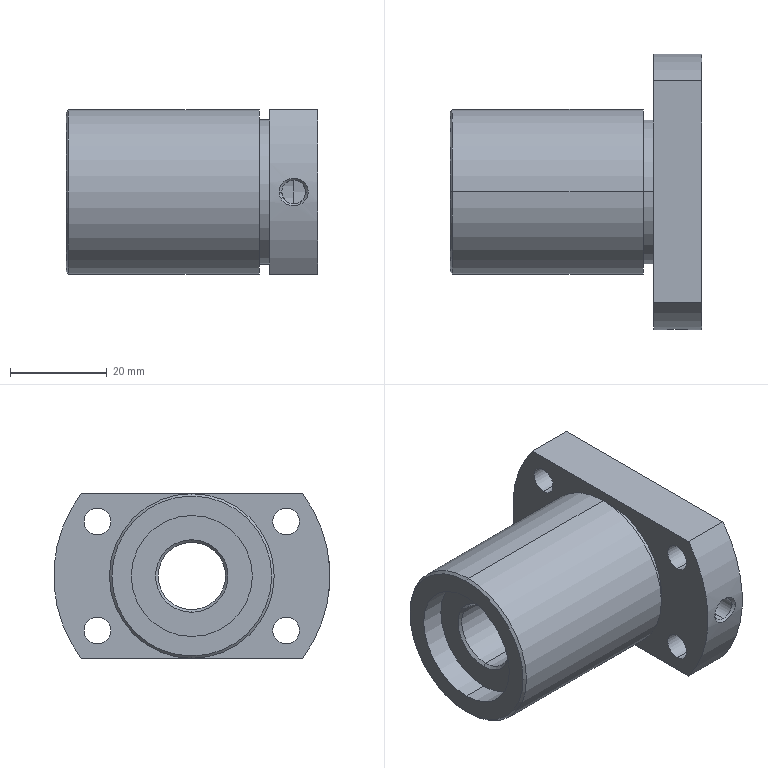Part | SolidWorks | features BaseBody 1 | 1 solid | 41 faces | box 52 x 57 x 34 mm | volume 42280 mm3 | cylinder 24 | plane 9 | cone 8 | commonest cylinder face diameters 5.5 x8 25 x4 4.917 x2 13.917 x2 21 x2 29.8 x2
STEP:
#1=CARTESIAN_POINT('',(39.9,0.,17.));
#2=VERTEX_POINT('',#1);
#3=CARTESIAN_POINT('',(39.9,0.,-17.));
#4=VERTEX_POINT('',#3);
#5=CARTESIAN_POINT('',(39.9,0.,0.));
#6=DIRECTION('',(-1.,0.,0.));
#7=DIRECTION('',(0.,0.,1.));
#8=AXIS2_PLACEMENT_3D('',#5,#6,#7);
#9=CIRCLE('',#8,17.);
#10=EDGE_CURVE('',#2,#4,#9,.T.);
#11=ORIENTED_EDGE('',*,*,#10,.T.);
#12=CARTESIAN_POINT('',(0.5,0.,-17.));
#13=VERTEX_POINT('',#12);
#14=CARTESIAN_POINT('',(42.,0.,-17.));
#15=DIRECTION('',(-1.,0.,0.));
#16=VECTOR('',#15,1000.);
#17=LINE('',#14,#16);
#18=EDGE_CURVE('',#4,#13,#17,.T.);
#19=ORIENTED_EDGE('',*,*,#18,.T.);
#20=CARTESIAN_POINT('',(0.5,0.,17.));
#21=VERTEX_POINT('',#20);
#22=CARTESIAN_POINT('',(0.5,0.,0.));
#23=DIRECTION('',(1.,0.,0.));
#24=DIRECTION('',(0.,0.,1.));
#25=AXIS2_PLACEMENT_3D('',#22,#23,#24);
#26=CIRCLE('',#25,17.);
#27=EDGE_CURVE('',#13,#21,#26,.T.);
#28=ORIENTED_EDGE('',*,*,#27,.T.);
#29=CARTESIAN_POINT('',(42.,0.,17.));
#30=DIRECTION('',(-1.,0.,0.));
#31=VECTOR('',#30,1000.);
#32=LINE('',#29,#31);
#33=EDGE_CURVE('',#2,#21,#32,.T.);
#34=ORIENTED_EDGE('',*,*,#33,.F.);
#35=EDGE_LOOP('',(#11,#19,#28,#34));
#36=FACE_OUTER_BOUND('',#35,.T.);
#37=CARTESIAN_POINT('',(42.,0.,0.));
#38=DIRECTION('',(-1.,0.,0.));
#39=DIRECTION('',(0.,0.,1.));
#40=AXIS2_PLACEMENT_3D('',#37,#38,#39);
#41=CYLINDRICAL_SURFACE('',#40,17.);
#42=ADVANCED_FACE('',(#36),#41,.T.);
#43=CARTESIAN_POINT('',(0.,0.,-16.5));
#44=VERTEX_POINT('',#43);
#45=CARTESIAN_POINT('',(0.,0.,16.5));
#46=VERTEX_POINT('',#45);
#47=CARTESIAN_POINT('',(0.,0.,0.));
#48=DIRECTION('',(1.,0.,0.));
#49=DIRECTION('',(0.,0.,-1.));
#50=AXIS2_PLACEMENT_3D('',#47,#48,#49);
#51=CIRCLE('',#50,16.5);
#52=EDGE_CURVE('',#44,#46,#51,.T.);
#53=ORIENTED_EDGE('',*,*,#52,.T.);
#54=CARTESIAN_POINT('',(0.5,0.,17.));
#55=DIRECTION('',(0.7071,0.,0.7071));
#56=VECTOR('',#55,1000.);
#57=LINE('',#54,#56);
#58=EDGE_CURVE('',#46,#21,#57,.T.);
#59=ORIENTED_EDGE('',*,*,#58,.T.);
#60=ORIENTED_EDGE('',*,*,#27,.F.);
#61=CARTESIAN_POINT('',(0.5,0.,-17.));
#62=DIRECTION('',(0.7071,0.,-0.7071));
#63=VECTOR('',#62,1000.);
#64=LINE('',#61,#63);
#65=EDGE_CURVE('',#44,#13,#64,.T.);
#66=ORIENTED_EDGE('',*,*,#65,.F.);
#67=EDGE_LOOP('',(#53,#59,#60,#66));
#68=FACE_OUTER_BOUND('',#67,.T.);
#69=CARTESIAN_POINT('',(0.5,0.,0.));
#70=DIRECTION('',(1.,0.,0.));
#71=DIRECTION('',(0.,0.,-1.));
#72=AXIS2_PLACEMENT_3D('',#69,#70,#71);
#73=CONICAL_SURFACE('',#72,17.,0.7854);
#74=ADVANCED_FACE('',(#68),#73,.T.);
#75=CARTESIAN_POINT('',(42.,0.,14.9));
#76=VERTEX_POINT('',#75);
#77=CARTESIAN_POINT('',(42.,0.,-14.9));
#78=VERTEX_POINT('',#77);
#79=CARTESIAN_POINT('',(42.,0.,0.));
#80=DIRECTION('',(-1.,0.,0.));
#81=DIRECTION('',(0.,0.,1.));
#82=AXIS2_PLACEMENT_3D('',#79,#80,#81);
#83=CIRCLE('',#82,14.9);
#84=EDGE_CURVE('',#76,#78,#83,.T.);
#85=ORIENTED_EDGE('',*,*,#84,.T.);
#86=CARTESIAN_POINT('',(39.9,0.,-14.9));
#87=VERTEX_POINT('',#86);
#88=CARTESIAN_POINT('',(42.,0.,-14.9));
#89=DIRECTION('',(-1.,0.,0.));
#90=VECTOR('',#89,1000.);
#91=LINE('',#88,#90);
#92=EDGE_CURVE('',#78,#87,#91,.T.);
#93=ORIENTED_EDGE('',*,*,#92,.T.);
#94=CARTESIAN_POINT('',(39.9,0.,14.9));
#95=VERTEX_POINT('',#94);
#96=CARTESIAN_POINT('',(39.9,0.,0.));
#97=DIRECTION('',(1.,0.,0.));
#98=DIRECTION('',(0.,0.,1.));
#99=AXIS2_PLACEMENT_3D('',#96,#97,#98);
#100=CIRCLE('',#99,14.9);
#101=EDGE_CURVE('',#87,#95,#100,.T.);
#102=ORIENTED_EDGE('',*,*,#101,.T.);
#103=CARTESIAN_POINT('',(42.,0.,14.9));
#104=DIRECTION('',(-1.,0.,0.));
#105=VECTOR('',#104,1000.);
#106=LINE('',#103,#105);
#107=EDGE_CURVE('',#76,#95,#106,.T.);
#108=ORIENTED_EDGE('',*,*,#107,.F.);
#109=EDGE_LOOP('',(#85,#93,#102,#108));
#110=FACE_OUTER_BOUND('',#109,.T.);
#111=CARTESIAN_POINT('',(42.,0.,0.));
#112=DIRECTION('',(-1.,0.,0.));
#113=DIRECTION('',(0.,0.,1.));
#114=AXIS2_PLACEMENT_3D('',#111,#112,#113);
#115=CYLINDRICAL_SURFACE('',#114,14.9);
#116=ADVANCED_FACE('',(#110),#115,.T.);
#117=CARTESIAN_POINT('',(5.,0.,-12.5));
#118=VERTEX_POINT('',#117);
#119=CARTESIAN_POINT('',(5.,0.,12.5));
#120=VERTEX_POINT('',#119);
#121=CARTESIAN_POINT('',(5.,0.,0.));
#122=DIRECTION('',(-1.,0.,0.));
#123=DIRECTION('',(0.,0.,1.));
#124=AXIS2_PLACEMENT_3D('',#121,#122,#123);
#125=CIRCLE('',#124,12.5);
#126=EDGE_CURVE('',#118,#120,#125,.T.);
#127=ORIENTED_EDGE('',*,*,#126,.F.);
#128=CARTESIAN_POINT('',(0.,0.,-12.5));
#129=VERTEX_POINT('',#128);
#130=CARTESIAN_POINT('',(52.,0.,-12.5));
#131=DIRECTION('',(-1.,0.,0.));
#132=VECTOR('',#131,1000.);
#133=LINE('',#130,#132);
#134=EDGE_CURVE('',#118,#129,#133,.T.);
#135=ORIENTED_EDGE('',*,*,#134,.T.);
#136=CARTESIAN_POINT('',(0.,0.,12.5));
#137=VERTEX_POINT('',#136);
#138=CARTESIAN_POINT('',(0.,0.,0.));
#139=DIRECTION('',(-1.,0.,0.));
#140=DIRECTION('',(0.,0.,1.));
#141=AXIS2_PLACEMENT_3D('',#138,#139,#140);
#142=CIRCLE('',#141,12.5);
#143=EDGE_CURVE('',#129,#137,#142,.T.);
#144=ORIENTED_EDGE('',*,*,#143,.T.);
#145=CARTESIAN_POINT('',(52.,0.,12.5));
#146=DIRECTION('',(-1.,0.,0.));
#147=VECTOR('',#146,1000.);
#148=LINE('',#145,#147);
#149=EDGE_CURVE('',#120,#137,#148,.T.);
#150=ORIENTED_EDGE('',*,*,#149,.F.);
#151=EDGE_LOOP('',(#127,#135,#144,#150));
#152=FACE_OUTER_BOUND('',#151,.T.);
#153=CARTESIAN_POINT('',(52.,0.,0.));
#154=DIRECTION('',(-1.,0.,0.));
#155=DIRECTION('',(0.,0.,1.));
#156=AXIS2_PLACEMENT_3D('',#153,#154,#155);
#157=CYLINDRICAL_SURFACE('',#156,12.5);
#158=ADVANCED_FACE('',(#152),#157,.F.);
#159=CARTESIAN_POINT('',(52.,19.486,8.5));
#160=VERTEX_POINT('',#159);
#161=CARTESIAN_POINT('',(52.,19.486,14.));
#162=VERTEX_POINT('',#161);
#163=CARTESIAN_POINT('',(52.,19.486,11.25));
#164=DIRECTION('',(-1.,0.,0.));
#165=DIRECTION('',(0.,0.,1.));
#166=AXIS2_PLACEMENT_3D('',#163,#164,#165);
#167=CIRCLE('',#166,2.75);
#168=EDGE_CURVE('',#160,#162,#167,.T.);
#169=ORIENTED_EDGE('',*,*,#168,.F.);
#170=CARTESIAN_POINT('',(42.,19.486,8.5));
#171=VERTEX_POINT('',#170);
#172=CARTESIAN_POINT('',(52.,19.486,8.5));
#173=DIRECTION('',(-1.,0.,0.));
#174=VECTOR('',#173,1000.);
#175=LINE('',#172,#174);
#176=EDGE_CURVE('',#160,#171,#175,.T.);
#177=ORIENTED_EDGE('',*,*,#176,.T.);
#178=CARTESIAN_POINT('',(42.,19.486,14.));
#179=VERTEX_POINT('',#178);
#180=CARTESIAN_POINT('',(42.,19.486,11.25));
#181=DIRECTION('',(-1.,0.,0.));
#182=DIRECTION('',(0.,0.,1.));
#183=AXIS2_PLACEMENT_3D('',#180,#181,#182);
#184=CIRCLE('',#183,2.75);
#185=EDGE_CURVE('',#171,#179,#184,.T.);
#186=ORIENTED_EDGE('',*,*,#185,.T.);
#187=CARTESIAN_POINT('',(52.,19.486,14.));
#188=DIRECTION('',(-1.,0.,0.));
#189=VECTOR('',#188,1000.);
#190=LINE('',#187,#189);
#191=EDGE_CURVE('',#162,#179,#190,.T.);
#192=ORIENTED_EDGE('',*,*,#191,.F.);
#193=EDGE_LOOP('',(#169,#177,#186,#192));
#194=FACE_OUTER_BOUND('',#193,.T.);
#195=CARTESIAN_POINT('',(52.,19.486,11.25));
#196=DIRECTION('',(-1.,0.,0.));
#197=DIRECTION('',(0.,0.,1.));
#198=AXIS2_PLACEMENT_3D('',#195,#196,#197);
#199=CYLINDRICAL_SURFACE('',#198,2.75);
#200=ADVANCED_FACE('',(#194),#199,.F.);
#201=CARTESIAN_POINT('',(52.,-19.486,-14.));
#202=VERTEX_POINT('',#201);
#203=CARTESIAN_POINT('',(52.,-19.486,-8.5));
#204=VERTEX_POINT('',#203);
#205=CARTESIAN_POINT('',(52.,-19.486,-11.25));
#206=DIRECTION('',(-1.,0.,0.));
#207=DIRECTION('',(0.,0.,1.));
#208=AXIS2_PLACEMENT_3D('',#205,#206,#207);
#209=CIRCLE('',#208,2.75);
#210=EDGE_CURVE('',#202,#204,#209,.T.);
#211=ORIENTED_EDGE('',*,*,#210,.F.);
#212=CARTESIAN_POINT('',(42.,-19.486,-14.));
#213=VERTEX_POINT('',#212);
#214=CARTESIAN_POINT('',(52.,-19.486,-14.));
#215=DIRECTION('',(-1.,0.,0.));
#216=VECTOR('',#215,1000.);
#217=LINE('',#214,#216);
#218=EDGE_CURVE('',#202,#213,#217,.T.);
#219=ORIENTED_EDGE('',*,*,#218,.T.);
#220=CARTESIAN_POINT('',(42.,-19.486,-8.5));
#221=VERTEX_POINT('',#220);
#222=CARTESIAN_POINT('',(42.,-19.486,-11.25));
#223=DIRECTION('',(-1.,0.,0.));
#224=DIRECTION('',(0.,0.,1.));
#225=AXIS2_PLACEMENT_3D('',#222,#223,#224);
#226=CIRCLE('',#225,2.75);
#227=EDGE_CURVE('',#213,#221,#226,.T.);
#228=ORIENTED_EDGE('',*,*,#227,.T.);
#229=CARTESIAN_POINT('',(52.,-19.486,-8.5));
#230=DIRECTION('',(-1.,0.,0.));
#231=VECTOR('',#230,1000.);
#232=LINE('',#229,#231);
#233=EDGE_CURVE('',#204,#221,#232,.T.);
#234=ORIENTED_EDGE('',*,*,#233,.F.);
#235=EDGE_LOOP('',(#211,#219,#228,#234));
#236=FACE_OUTER_BOUND('',#235,.T.);
#237=CARTESIAN_POINT('',(52.,-19.486,-11.25));
#238=DIRECTION('',(-1.,0.,0.));
#239=DIRECTION('',(0.,0.,1.));
#240=AXIS2_PLACEMENT_3D('',#237,#238,#239);
#241=CYLINDRICAL_SURFACE('',#240,2.75);
#242=ADVANCED_FACE('',(#236),#241,.F.);
#243=CARTESIAN_POINT('',(52.,19.486,-14.));
#244=VERTEX_POINT('',#243);
#245=CARTESIAN_POINT('',(52.,19.486,-8.5));
#246=VERTEX_POINT('',#245);
#247=CARTESIAN_POINT('',(52.,19.486,-11.25));
#248=DIRECTION('',(-1.,0.,0.));
#249=DIRECTION('',(0.,0.,1.));
#250=AXIS2_PLACEMENT_3D('',#247,#248,#249);
#251=CIRCLE('',#250,2.75);
#252=EDGE_CURVE('',#244,#246,#251,.T.);
#253=ORIENTED_EDGE('',*,*,#252,.F.);
#254=CARTESIAN_POINT('',(42.,19.486,-14.));
#255=VERTEX_POINT('',#254);
#256=CARTESIAN_POINT('',(52.,19.486,-14.));
#257=DIRECTION('',(-1.,0.,0.));
#258=VECTOR('',#257,1000.);
#259=LINE('',#256,#258);
#260=EDGE_CURVE('',#244,#255,#259,.T.);
#261=ORIENTED_EDGE('',*,*,#260,.T.);
#262=CARTESIAN_POINT('',(42.,19.486,-8.5));
#263=VERTEX_POINT('',#262);
#264=CARTESIAN_POINT('',(42.,19.486,-11.25));
#265=DIRECTION('',(-1.,0.,0.));
#266=DIRECTION('',(0.,0.,1.));
#267=AXIS2_PLACEMENT_3D('',#264,#265,#266);
#268=CIRCLE('',#267,2.75);
#269=EDGE_CURVE('',#255,#263,#268,.T.);
#270=ORIENTED_EDGE('',*,*,#269,.T.);
#271=CARTESIAN_POINT('',(52.,19.486,-8.5));
#272=DIRECTION('',(-1.,0.,0.));
#273=VECTOR('',#272,1000.);
#274=LINE('',#271,#273);
#275=EDGE_CURVE('',#246,#263,#274,.T.);
#276=ORIENTED_EDGE('',*,*,#275,.F.);
#277=EDGE_LOOP('',(#253,#261,#270,#276));
#278=FACE_OUTER_BOUND('',#277,.T.);
#279=CARTESIAN_POINT('',(52.,19.486,-11.25));
#280=DIRECTION('',(-1.,0.,0.));
#281=DIRECTION('',(0.,0.,1.));
#282=AXIS2_PLACEMENT_3D('',#279,#280,#281);
#283=CYLINDRICAL_SURFACE('',#282,2.75);
#284=ADVANCED_FACE('',(#278),#283,.F.);
#285=CARTESIAN_POINT('',(52.,-19.486,8.5));
#286=VERTEX_POINT('',#285);
#287=CARTESIAN_POINT('',(52.,-19.486,14.));
#288=VERTEX_POINT('',#287);
#289=CARTESIAN_POINT('',(52.,-19.486,11.25));
#290=DIRECTION('',(-1.,0.,0.));
#291=DIRECTION('',(0.,0.,1.));
#292=AXIS2_PLACEMENT_3D('',#289,#290,#291);
#293=CIRCLE('',#292,2.75);
#294=EDGE_CURVE('',#286,#288,#293,.T.);
#295=ORIENTED_EDGE('',*,*,#294,.F.);
#296=CARTESIAN_POINT('',(42.,-19.486,8.5));
#297=VERTEX_POINT('',#296);
#298=CARTESIAN_POINT('',(52.,-19.486,8.5));
#299=DIRECTION('',(-1.,0.,0.));
#300=VECTOR('',#299,1000.);
#301=LINE('',#298,#300);
#302=EDGE_CURVE('',#286,#297,#301,.T.);
#303=ORIENTED_EDGE('',*,*,#302,.T.);
#304=CARTESIAN_POINT('',(42.,-19.486,14.));
#305=VERTEX_POINT('',#304);
#306=CARTESIAN_POINT('',(42.,-19.486,11.25));
#307=DIRECTION('',(-1.,0.,0.));
#308=DIRECTION('',(0.,0.,1.));
#309=AXIS2_PLACEMENT_3D('',#306,#307,#308);
#310=CIRCLE('',#309,2.75);
#311=EDGE_CURVE('',#297,#305,#310,.T.);
#312=ORIENTED_EDGE('',*,*,#311,.T.);
#313=CARTESIAN_POINT('',(52.,-19.486,14.));
#314=DIRECTION('',(-1.,0.,0.));
#315=VECTOR('',#314,1000.);
#316=LINE('',#313,#315);
#317=EDGE_CURVE('',#288,#305,#316,.T.);
#318=ORIENTED_EDGE('',*,*,#317,.F.);
#319=EDGE_LOOP('',(#295,#303,#312,#318));
#320=FACE_OUTER_BOUND('',#319,.T.);
#321=CARTESIAN_POINT('',(52.,-19.486,11.25));
#322=DIRECTION('',(-1.,0.,0.));
#323=DIRECTION('',(0.,0.,1.));
#324=AXIS2_PLACEMENT_3D('',#321,#322,#323);
#325=CYLINDRICAL_SURFACE('',#324,2.75);
#326=ADVANCED_FACE('',(#320),#325,.F.);
#327=CARTESIAN_POINT('',(5.542,0.,-6.958));
#328=VERTEX_POINT('',#327);
#329=CARTESIAN_POINT('',(5.542,0.,6.958));
#330=VERTEX_POINT('',#329);
#331=CARTESIAN_POINT('',(5.542,0.,0.));
#332=DIRECTION('',(-1.,0.,0.));
#333=DIRECTION('',(0.,0.,1.));
#334=AXIS2_PLACEMENT_3D('',#331,#332,#333);
#335=CIRCLE('',#334,6.958);
#336=EDGE_CURVE('',#328,#330,#335,.T.);
#337=ORIENTED_EDGE('',*,*,#336,.F.);
#338=CARTESIAN_POINT('',(5.,0.,-7.5));
#339=VERTEX_POINT('',#338);
#340=CARTESIAN_POINT('',(5.,0.,-7.5));
#341=DIRECTION('',(-0.7071,0.,-0.7071));
#342=VECTOR('',#341,1000.);
#343=LINE('',#340,#342);
#344=EDGE_CURVE('',#328,#339,#343,.T.);
#345=ORIENTED_EDGE('',*,*,#344,.T.);
#346=CARTESIAN_POINT('',(5.,0.,7.5));
#347=VERTEX_POINT('',#346);
#348=CARTESIAN_POINT('',(5.,0.,0.));
#349=DIRECTION('',(1.,0.,0.));
#350=DIRECTION('',(0.,0.,1.));
#351=AXIS2_PLACEMENT_3D('',#348,#349,#350);
#352=CIRCLE('',#351,7.5);
#353=EDGE_CURVE('',#347,#339,#352,.T.);
#354=ORIENTED_EDGE('',*,*,#353,.F.);
#355=CARTESIAN_POINT('',(5.,0.,7.5));
#356=DIRECTION('',(-0.7071,0.,0.7071));
#357=VECTOR('',#356,1000.);
#358=LINE('',#355,#357);
#359=EDGE_CURVE('',#330,#347,#358,.T.);
#360=ORIENTED_EDGE('',*,*,#359,.F.);
#361=EDGE_LOOP('',(#337,#345,#354,#360));
#362=FACE_OUTER_BOUND('',#361,.T.);
#363=CARTESIAN_POINT('',(5.,0.,0.));
#364=DIRECTION('',(-1.,0.,0.));
#365=DIRECTION('',(0.,0.,1.));
#366=AXIS2_PLACEMENT_3D('',#363,#364,#365);
#367=CONICAL_SURFACE('',#366,7.5,0.7854);
#368=ADVANCED_FACE('',(#362),#367,.F.);
#369=CARTESIAN_POINT('',(44.542,-27.958,0.));
#370=VERTEX_POINT('',#369);
#371=CARTESIAN_POINT('',(47.,-27.958,-2.458));
#372=VERTEX_POINT('',#371);
#373=CARTESIAN_POINT('',(47.,-27.958,0.));
#374=DIRECTION('',(0.,-1.,0.));
#375=DIRECTION('',(0.,0.,-1.));
#376=AXIS2_PLACEMENT_3D('',#373,#374,#375);
#377=CIRCLE('',#376,2.458);
#378=EDGE_CURVE('',#370,#372,#377,.T.);
#379=ORIENTED_EDGE('',*,*,#378,.F.);
#380=CARTESIAN_POINT('',(44.,-28.5,0.));
#381=VERTEX_POINT('',#380);
#382=CARTESIAN_POINT('',(43.997,-28.503,0.));
#383=DIRECTION('',(-0.7071,-0.7071,0.));
#384=VECTOR('',#383,1000.);
#385=LINE('',#382,#384);
#386=EDGE_CURVE('',#370,#381,#385,.T.);
#387=ORIENTED_EDGE('',*,*,#386,.T.);
#388=CARTESIAN_POINT('',(50.,-28.5,0.));
#389=VERTEX_POINT('',#388);
#390=CARTESIAN_POINT('',(50.,-28.5,0.));
#391=CARTESIAN_POINT('',(50.,-28.5,-0.1909));
#392=CARTESIAN_POINT('',(49.98,-28.498,-0.384));
#393=CARTESIAN_POINT('',(49.899,-28.49,-0.7601));
#394=CARTESIAN_POINT('',(49.839,-28.485,-0.9415));
#395=CARTESIAN_POINT('',(49.683,-28.471,-1.292));
#396=CARTESIAN_POINT('',(49.585,-28.463,-1.46));
#397=CARTESIAN_POINT('',(49.362,-28.445,-1.77));
#398=CARTESIAN_POINT('',(49.235,-28.436,-1.914));
#399=CARTESIAN_POINT('',(48.952,-28.417,-2.177));
#400=CARTESIAN_POINT('',(48.8,-28.408,-2.292));
#401=CARTESIAN_POINT('',(48.475,-28.391,-2.494));
#402=CARTESIAN_POINT('',(48.301,-28.383,-2.58));
#403=CARTESIAN_POINT('',(47.943,-28.37,-2.718));
#404=CARTESIAN_POINT('',(47.759,-28.365,-2.769));
#405=CARTESIAN_POINT('',(47.382,-28.358,-2.839));
#406=CARTESIAN_POINT('',(47.188,-28.356,-2.857));
#407=CARTESIAN_POINT('',(46.802,-28.357,-2.856));
#408=CARTESIAN_POINT('',(46.611,-28.358,-2.838));
#409=CARTESIAN_POINT('',(46.237,-28.365,-2.768));
#410=CARTESIAN_POINT('',(46.051,-28.37,-2.716));
#411=CARTESIAN_POINT('',(45.692,-28.383,-2.577));
#412=CARTESIAN_POINT('',(45.521,-28.391,-2.492));
#413=CARTESIAN_POINT('',(45.198,-28.408,-2.29));
#414=CARTESIAN_POINT('',(45.043,-28.417,-2.172));
#415=CARTESIAN_POINT('',(44.763,-28.436,-1.911));
#416=CARTESIAN_POINT('',(44.637,-28.445,-1.769));
#417=CARTESIAN_POINT('',(44.414,-28.463,-1.459));
#418=CARTESIAN_POINT('',(44.316,-28.471,-1.29));
#419=CARTESIAN_POINT('',(44.161,-28.485,-0.9409));
#420=CARTESIAN_POINT('',(44.101,-28.49,-0.7598));
#421=CARTESIAN_POINT('',(44.02,-28.498,-0.3831));
#422=CARTESIAN_POINT('',(44.,-28.5,-0.1908));
#423=CARTESIAN_POINT('',(44.,-28.5,0.));
#424=B_SPLINE_CURVE_WITH_KNOTS('',3,(#390,#391,#392,#393,#394,#395,#396,#397,#398,#399,#400,#401,#402,#403,#404,#405,#406,#407,#408,#409,#410,#411,#412,#413,#414,#415,#416,#417,#418,#419,#420,#421,#422,#423),.UNSPECIFIED.,.F.,.F.,(4,2,2,2,2,2,2,2,2,2,2,2,2,2,2,2,4),(0.01373,0.0143,0.01488,0.01545,0.01602,0.01659,0.01716,0.01774,0.01831,0.01888,0.01945,0.02002,0.0206,0.02117,0.02174,0.02231,0.02288),.UNSPECIFIED.);
#425=EDGE_CURVE('',#389,#381,#424,.T.);
#426=ORIENTED_EDGE('',*,*,#425,.F.);
#427=CARTESIAN_POINT('',(49.458,-27.958,0.));
#428=VERTEX_POINT('',#427);
#429=CARTESIAN_POINT('',(50.003,-28.503,0.));
#430=DIRECTION('',(0.7071,-0.7071,0.));
#431=VECTOR('',#430,1000.);
#432=LINE('',#429,#431);
#433=EDGE_CURVE('',#428,#389,#432,.T.);
#434=ORIENTED_EDGE('',*,*,#433,.F.);
#435=CARTESIAN_POINT('',(47.,-27.958,0.));
#436=DIRECTION('',(0.,-1.,0.));
#437=DIRECTION('',(0.,0.,-1.));
#438=AXIS2_PLACEMENT_3D('',#435,#436,#437);
#439=CIRCLE('',#438,2.458);
#440=EDGE_CURVE('',#372,#428,#439,.T.);
#441=ORIENTED_EDGE('',*,*,#440,.F.);
#442=EDGE_LOOP('',(#379,#387,#426,#434,#441));
#443=FACE_OUTER_BOUND('',#442,.T.);
#444=CARTESIAN_POINT('',(47.,-28.503,0.));
#445=DIRECTION('',(0.,-1.,0.));
#446=DIRECTION('',(1.,0.,0.));
#447=AXIS2_PLACEMENT_3D('',#444,#445,#446);
#448=CONICAL_SURFACE('',#447,3.003,0.7854);
#449=ADVANCED_FACE('',(#443),#448,.F.);
#450=CARTESIAN_POINT('',(41.459,0.,-6.958));
#451=VERTEX_POINT('',#450);
#452=CARTESIAN_POINT('',(41.459,0.,6.958));
#453=VERTEX_POINT('',#452);
#454=CARTESIAN_POINT('',(41.459,0.,0.));
#455=DIRECTION('',(-1.,0.,0.));
#456=DIRECTION('',(0.,0.,1.));
#457=AXIS2_PLACEMENT_3D('',#454,#455,#456);
#458=CIRCLE('',#457,6.958);
#459=EDGE_CURVE('',#451,#453,#458,.T.);
#460=ORIENTED_EDGE('',*,*,#459,.F.);
#461=CARTESIAN_POINT('',(52.,0.,-6.958));
#462=DIRECTION('',(-1.,0.,0.));
#463=VECTOR('',#462,1000.);
#464=LINE('',#461,#463);
#465=EDGE_CURVE('',#451,#328,#464,.T.);
#466=ORIENTED_EDGE('',*,*,#465,.T.);
#467=ORIENTED_EDGE('',*,*,#336,.T.);
#468=CARTESIAN_POINT('',(52.,0.,6.958));
#469=DIRECTION('',(-1.,0.,0.));
#470=VECTOR('',#469,1000.);
#471=LINE('',#468,#470);
#472=EDGE_CURVE('',#453,#330,#471,.T.);
#473=ORIENTED_EDGE('',*,*,#472,.F.);
#474=EDGE_LOOP('',(#460,#466,#467,#473));
#475=FACE_OUTER_BOUND('',#474,.T.);
#476=CARTESIAN_POINT('',(52.,0.,0.));
#477=DIRECTION('',(-1.,0.,0.));
#478=DIRECTION('',(0.,0.,1.));
#479=AXIS2_PLACEMENT_3D('',#476,#477,#478);
#480=CYLINDRICAL_SURFACE('',#479,6.958);
#481=ADVANCED_FACE('',(#475),#480,.F.);
#482=CARTESIAN_POINT('',(52.,0.,-12.5));
#483=VERTEX_POINT('',#482);
#484=CARTESIAN_POINT('',(52.,0.,12.5));
#485=VERTEX_POINT('',#484);
#486=CARTESIAN_POINT('',(52.,0.,0.));
#487=DIRECTION('',(-1.,0.,0.));
#488=DIRECTION('',(0.,0.,1.));
#489=AXIS2_PLACEMENT_3D('',#486,#487,#488);
#490=CIRCLE('',#489,12.5);
#491=EDGE_CURVE('',#483,#485,#490,.T.);
#492=ORIENTED_EDGE('',*,*,#491,.F.);
#493=CARTESIAN_POINT('',(47.,0.,-12.5));
#494=VERTEX_POINT('',#493);
#495=CARTESIAN_POINT('',(52.,0.,-12.5));
#496=DIRECTION('',(-1.,0.,0.));
#497=VECTOR('',#496,1000.);
#498=LINE('',#495,#497);
#499=EDGE_CURVE('',#483,#494,#498,.T.);
#500=ORIENTED_EDGE('',*,*,#499,.T.);
#501=CARTESIAN_POINT('',(47.,-12.256,-2.459));
#502=VERTEX_POINT('',#501);
#503=CARTESIAN_POINT('',(47.,0.,0.));
#504=DIRECTION('',(1.,0.,0.));
#505=DIRECTION('',(0.,0.,1.));
#506=AXIS2_PLACEMENT_3D('',#503,#504,#505);
#507=CIRCLE('',#506,12.5);
#508=EDGE_CURVE('',#502,#494,#507,.T.);
#509=ORIENTED_EDGE('',*,*,#508,.F.);
#510=CARTESIAN_POINT('',(47.,-12.256,2.459));
#511=VERTEX_POINT('',#510);
#512=CARTESIAN_POINT('',(47.,-12.256,2.459));
#513=CARTESIAN_POINT('',(47.163,-12.256,2.459));
#514=CARTESIAN_POINT('',(47.323,-12.259,2.442));
#515=CARTESIAN_POINT('',(47.638,-12.271,2.38));
#516=CARTESIAN_POINT('',(47.794,-12.281,2.332));
#517=CARTESIAN_POINT('',(48.091,-12.303,2.209));
#518=CARTESIAN_POINT('',(48.232,-12.317,2.133));
#519=CARTESIAN_POINT('',(48.499,-12.347,1.955));
#520=CARTESIAN_POINT('',(48.625,-12.363,1.851));
#521=CARTESIAN_POINT('',(48.965,-12.41,1.512));
#522=CARTESIAN_POINT('',(49.148,-12.442,1.239));
#523=CARTESIAN_POINT('',(49.332,-12.476,0.7953));
#524=CARTESIAN_POINT('',(49.379,-12.485,0.64));
#525=CARTESIAN_POINT('',(49.443,-12.497,0.3225));
#526=CARTESIAN_POINT('',(49.458,-12.5,0.1627));
#527=CARTESIAN_POINT('',(49.459,-12.5,-0.1588));
#528=CARTESIAN_POINT('',(49.443,-12.497,-0.3221));
#529=CARTESIAN_POINT('',(49.38,-12.485,-0.6377));
#530=CARTESIAN_POINT('',(49.333,-12.476,-0.7911));
#531=CARTESIAN_POINT('',(49.21,-12.453,-1.089));
#532=CARTESIAN_POINT('',(49.133,-12.44,-1.233));
#533=CARTESIAN_POINT('',(48.956,-12.411,-1.499));
#534=CARTESIAN_POINT('',(48.854,-12.395,-1.623));
#535=CARTESIAN_POINT('',(48.625,-12.363,-1.852));
#536=CARTESIAN_POINT('',(48.501,-12.347,-1.953));
#537=CARTESIAN_POINT('',(48.236,-12.317,-2.131));
#538=CARTESIAN_POINT('',(48.092,-12.303,-2.209));
#539=CARTESIAN_POINT('',(47.795,-12.281,-2.332));
#540=CARTESIAN_POINT('',(47.642,-12.272,-2.379));
#541=CARTESIAN_POINT('',(47.326,-12.259,-2.442));
#542=CARTESIAN_POINT('',(47.163,-12.256,-2.459));
#543=CARTESIAN_POINT('',(47.,-12.256,-2.459));
#544=B_SPLINE_CURVE_WITH_KNOTS('',3,(#512,#513,#514,#515,#516,#517,#518,#519,#520,#521,#522,#523,#524,#525,#526,#527,#528,#529,#530,#531,#532,#533,#534,#535,#536,#537,#538,#539,#540,#541,#542,#543),.UNSPECIFIED.,.F.,.F.,(4,2,2,2,2,2,2,2,2,2,2,2,2,2,2,4),(0.,0.0004814,0.0009629,0.001444,0.001926,0.002889,0.00337,0.003852,0.004333,0.004814,0.005296,0.005777,0.006259,0.00674,0.007222,0.007703),.UNSPECIFIED.);
#545=EDGE_CURVE('',#511,#502,#544,.T.);
#546=ORIENTED_EDGE('',*,*,#545,.F.);
#547=CARTESIAN_POINT('',(47.,0.,12.5));
#548=VERTEX_POINT('',#547);
#549=CARTESIAN_POINT('',(47.,0.,0.));
#550=DIRECTION('',(1.,0.,0.));
#551=DIRECTION('',(0.,0.,1.));
#552=AXIS2_PLACEMENT_3D('',#549,#550,#551);
#553=CIRCLE('',#552,12.5);
#554=EDGE_CURVE('',#548,#511,#553,.T.);
#555=ORIENTED_EDGE('',*,*,#554,.F.);
#556=CARTESIAN_POINT('',(52.,0.,12.5));
#557=DIRECTION('',(-1.,0.,0.));
#558=VECTOR('',#557,1000.);
#559=LINE('',#556,#558);
#560=EDGE_CURVE('',#485,#548,#559,.T.);
#561=ORIENTED_EDGE('',*,*,#560,.F.);
#562=EDGE_LOOP('',(#492,#500,#509,#546,#555,#561));
#563=FACE_OUTER_BOUND('',#562,.T.);
#564=CARTESIAN_POINT('',(52.,0.,0.));
#565=DIRECTION('',(-1.,0.,0.));
#566=DIRECTION('',(0.,0.,1.));
#567=AXIS2_PLACEMENT_3D('',#564,#565,#566);
#568=CYLINDRICAL_SURFACE('',#567,12.5);
#569=ADVANCED_FACE('',(#563),#568,.F.);
#570=CARTESIAN_POINT('',(47.,-27.958,2.458));
#571=VERTEX_POINT('',#570);
#572=CARTESIAN_POINT('',(47.,-27.958,0.));
#573=DIRECTION('',(0.,-1.,0.));
#574=DIRECTION('',(0.,0.,-1.));
#575=AXIS2_PLACEMENT_3D('',#572,#573,#574);
#576=CIRCLE('',#575,2.458);
#577=EDGE_CURVE('',#571,#370,#576,.T.);
#578=ORIENTED_EDGE('',*,*,#577,.T.);
#579=ORIENTED_EDGE('',*,*,#378,.T.);
#580=CARTESIAN_POINT('',(47.,-28.5,-2.459));
#581=DIRECTION('',(0.,1.,0.));
#582=VECTOR('',#581,1000.);
#583=LINE('',#580,#582);
#584=EDGE_CURVE('',#372,#502,#583,.T.);
#585=ORIENTED_EDGE('',*,*,#584,.T.);
#586=CARTESIAN_POINT('',(47.,-10.208,-2.459));
#587=VERTEX_POINT('',#586);
#588=CARTESIAN_POINT('',(47.,-28.5,-2.459));
#589=DIRECTION('',(0.,-1.,0.));
#590=VECTOR('',#589,1000.);
#591=LINE('',#588,#590);
#592=EDGE_CURVE('',#587,#502,#591,.T.);
#593=ORIENTED_EDGE('',*,*,#592,.F.);
#594=CARTESIAN_POINT('',(47.,-10.208,2.459));
#595=VERTEX_POINT('',#594);
#596=CARTESIAN_POINT('',(47.,-10.208,2.459));
#597=CARTESIAN_POINT('',(46.837,-10.208,2.459));
#598=CARTESIAN_POINT('',(46.677,-10.212,2.442));
#599=CARTESIAN_POINT('',(46.362,-10.227,2.38));
#600=CARTESIAN_POINT('',(46.206,-10.238,2.332));
#601=CARTESIAN_POINT('',(45.908,-10.265,2.209));
#602=CARTESIAN_POINT('',(45.767,-10.281,2.133));
#603=CARTESIAN_POINT('',(45.5,-10.317,1.955));
#604=CARTESIAN_POINT('',(45.375,-10.336,1.851));
#605=CARTESIAN_POINT('',(45.036,-10.393,1.513));
#606=CARTESIAN_POINT('',(44.853,-10.431,1.239));
#607=CARTESIAN_POINT('',(44.668,-10.471,0.796));
#608=CARTESIAN_POINT('',(44.621,-10.482,0.6405));
#609=CARTESIAN_POINT('',(44.557,-10.496,0.3229));
#610=CARTESIAN_POINT('',(44.542,-10.5,0.1631));
#611=CARTESIAN_POINT('',(44.541,-10.5,-0.1588));
#612=CARTESIAN_POINT('',(44.557,-10.496,-0.3223));
#613=CARTESIAN_POINT('',(44.62,-10.482,-0.6381));
#614=CARTESIAN_POINT('',(44.667,-10.471,-0.7916));
#615=CARTESIAN_POINT('',(44.852,-10.431,-1.239));
#616=CARTESIAN_POINT('',(45.033,-10.393,-1.51));
#617=CARTESIAN_POINT('',(45.375,-10.336,-1.852));
#618=CARTESIAN_POINT('',(45.498,-10.317,-1.953));
#619=CARTESIAN_POINT('',(45.764,-10.282,-2.131));
#620=CARTESIAN_POINT('',(45.908,-10.265,-2.208));
#621=CARTESIAN_POINT('',(46.204,-10.238,-2.332));
#622=CARTESIAN_POINT('',(46.358,-10.227,-2.379));
#623=CARTESIAN_POINT('',(46.674,-10.212,-2.442));
#624=CARTESIAN_POINT('',(46.837,-10.208,-2.459));
#625=CARTESIAN_POINT('',(47.,-10.208,-2.459));
#626=B_SPLINE_CURVE_WITH_KNOTS('',3,(#596,#597,#598,#599,#600,#601,#602,#603,#604,#605,#606,#607,#608,#609,#610,#611,#612,#613,#614,#615,#616,#617,#618,#619,#620,#621,#622,#623,#624,#625),.UNSPECIFIED.,.F.,.F.,(4,2,2,2,2,2,2,2,2,2,2,2,2,2,4),(0.,0.0004819,0.0009639,0.001446,0.001928,0.002892,0.003374,0.003855,0.004337,0.004819,0.005783,0.006265,0.006747,0.007229,0.007711),.UNSPECIFIED.);
#627=EDGE_CURVE('',#595,#587,#626,.T.);
#628=ORIENTED_EDGE('',*,*,#627,.F.);
#629=CARTESIAN_POINT('',(47.,-28.5,2.459));
#630=DIRECTION('',(0.,1.,0.));
#631=VECTOR('',#630,1000.);
#632=LINE('',#629,#631);
#633=EDGE_CURVE('',#511,#595,#632,.T.);
#634=ORIENTED_EDGE('',*,*,#633,.F.);
#635=CARTESIAN_POINT('',(47.,-28.5,2.459));
#636=DIRECTION('',(0.,1.,0.));
#637=VECTOR('',#636,1000.);
#638=LINE('',#635,#637);
#639=EDGE_CURVE('',#571,#511,#638,.T.);
#640=ORIENTED_EDGE('',*,*,#639,.F.);
#641=EDGE_LOOP('',(#578,#579,#585,#593,#628,#634,#640));
#642=FACE_OUTER_BOUND('',#641,.T.);
#643=CARTESIAN_POINT('',(47.,-28.5,0.));
#644=DIRECTION('',(0.,1.,0.));
#645=DIRECTION('',(0.,0.,1.));
#646=AXIS2_PLACEMENT_3D('',#643,#644,#645);
#647=CYLINDRICAL_SURFACE('',#646,2.459);
#648=ADVANCED_FACE('',(#642),#647,.F.);
#649=ORIENTED_EDGE('',*,*,#459,.T.);
#650=CARTESIAN_POINT('',(42.,0.,7.5));
#651=VERTEX_POINT('',#650);
#652=CARTESIAN_POINT('',(42.,0.,7.5));
#653=DIRECTION('',(0.7071,0.,0.7071));
#654=VECTOR('',#653,1000.);
#655=LINE('',#652,#654);
#656=EDGE_CURVE('',#453,#651,#655,.T.);
#657=ORIENTED_EDGE('',*,*,#656,.T.);
#658=CARTESIAN_POINT('',(42.,0.,-7.5));
#659=VERTEX_POINT('',#658);
#660=CARTESIAN_POINT('',(42.,0.,0.));
#661=DIRECTION('',(-1.,0.,0.));
#662=DIRECTION('',(0.,0.,-1.));
#663=AXIS2_PLACEMENT_3D('',#660,#661,#662);
#664=CIRCLE('',#663,7.5);
#665=EDGE_CURVE('',#659,#651,#664,.T.);
#666=ORIENTED_EDGE('',*,*,#665,.F.);
#667=CARTESIAN_POINT('',(42.,0.,-7.5));
#668=DIRECTION('',(0.7071,0.,-0.7071));
#669=VECTOR('',#668,1000.);
#670=LINE('',#667,#669);
#671=EDGE_CURVE('',#451,#659,#670,.T.);
#672=ORIENTED_EDGE('',*,*,#671,.F.);
#673=EDGE_LOOP('',(#649,#657,#666,#672));
#674=FACE_OUTER_BOUND('',#673,.T.);
#675=CARTESIAN_POINT('',(42.,0.,0.));
#676=DIRECTION('',(1.,0.,0.));
#677=DIRECTION('',(0.,0.,-1.));
#678=AXIS2_PLACEMENT_3D('',#675,#676,#677);
#679=CONICAL_SURFACE('',#678,7.5,0.7854);
#680=ADVANCED_FACE('',(#674),#679,.F.);
#681=CARTESIAN_POINT('',(47.,0.,-10.5));
#682=VERTEX_POINT('',#681);
#683=CARTESIAN_POINT('',(47.,0.,0.));
#684=DIRECTION('',(-1.,0.,0.));
#685=DIRECTION('',(0.,0.,1.));
#686=AXIS2_PLACEMENT_3D('',#683,#684,#685);
#687=CIRCLE('',#686,10.5);
#688=EDGE_CURVE('',#682,#587,#687,.T.);
#689=ORIENTED_EDGE('',*,*,#688,.F.);
#690=CARTESIAN_POINT('',(42.,0.,-10.5));
#691=VERTEX_POINT('',#690);
#692=CARTESIAN_POINT('',(52.,0.,-10.5));
#693=DIRECTION('',(-1.,0.,0.));
#694=VECTOR('',#693,1000.);
#695=LINE('',#692,#694);
#696=EDGE_CURVE('',#682,#691,#695,.T.);
#697=ORIENTED_EDGE('',*,*,#696,.T.);
#698=CARTESIAN_POINT('',(42.,0.,10.5));
#699=VERTEX_POINT('',#698);
#700=CARTESIAN_POINT('',(42.,0.,0.));
#701=DIRECTION('',(1.,0.,0.));
#702=DIRECTION('',(0.,0.,1.));
#703=AXIS2_PLACEMENT_3D('',#700,#701,#702);
#704=CIRCLE('',#703,10.5);
#705=EDGE_CURVE('',#699,#691,#704,.T.);
#706=ORIENTED_EDGE('',*,*,#705,.F.);
#707=CARTESIAN_POINT('',(47.,0.,10.5));
#708=VERTEX_POINT('',#707);
#709=CARTESIAN_POINT('',(52.,0.,10.5));
#710=DIRECTION('',(-1.,0.,0.));
#711=VECTOR('',#710,1000.);
#712=LINE('',#709,#711);
#713=EDGE_CURVE('',#708,#699,#712,.T.);
#714=ORIENTED_EDGE('',*,*,#713,.F.);
#715=CARTESIAN_POINT('',(47.,0.,0.));
#716=DIRECTION('',(-1.,0.,0.));
#717=DIRECTION('',(0.,0.,1.));
#718=AXIS2_PLACEMENT_3D('',#715,#716,#717);
#719=CIRCLE('',#718,10.5);
#720=EDGE_CURVE('',#595,#708,#719,.T.);
#721=ORIENTED_EDGE('',*,*,#720,.F.);
#722=ORIENTED_EDGE('',*,*,#627,.T.);
#723=EDGE_LOOP('',(#689,#697,#706,#714,#721,#722));
#724=FACE_OUTER_BOUND('',#723,.T.);
#725=CARTESIAN_POINT('',(52.,0.,0.));
#726=DIRECTION('',(-1.,0.,0.));
#727=DIRECTION('',(0.,0.,1.));
#728=AXIS2_PLACEMENT_3D('',#725,#726,#727);
#729=CYLINDRICAL_SURFACE('',#728,10.5);
#730=ADVANCED_FACE('',(#724),#729,.F.);
#731=ORIENTED_EDGE('',*,*,#18,.F.);
#732=CARTESIAN_POINT('',(39.9,0.,0.));
#733=DIRECTION('',(-1.,0.,0.));
#734=DIRECTION('',(0.,0.,1.));
#735=AXIS2_PLACEMENT_3D('',#732,#733,#734);
#736=CIRCLE('',#735,17.);
#737=EDGE_CURVE('',#4,#2,#736,.T.);
#738=ORIENTED_EDGE('',*,*,#737,.T.);
#739=ORIENTED_EDGE('',*,*,#33,.T.);
#740=CARTESIAN_POINT('',(0.5,0.,0.));
#741=DIRECTION('',(1.,0.,0.));
#742=DIRECTION('',(0.,0.,1.));
#743=AXIS2_PLACEMENT_3D('',#740,#741,#742);
#744=CIRCLE('',#743,17.);
#745=EDGE_CURVE('',#21,#13,#744,.T.);
#746=ORIENTED_EDGE('',*,*,#745,.T.);
#747=EDGE_LOOP('',(#731,#738,#739,#746));
#748=FACE_OUTER_BOUND('',#747,.T.);
#749=CARTESIAN_POINT('',(42.,0.,0.));
#750=DIRECTION('',(-1.,0.,0.));
#751=DIRECTION('',(0.,0.,1.));
#752=AXIS2_PLACEMENT_3D('',#749,#750,#751);
#753=CYLINDRICAL_SURFACE('',#752,17.);
#754=ADVANCED_FACE('',(#748),#753,.T.);
#755=ORIENTED_EDGE('',*,*,#58,.F.);
#756=CARTESIAN_POINT('',(0.,0.,0.));
#757=DIRECTION('',(1.,0.,0.));
#758=DIRECTION('',(0.,0.,-1.));
#759=AXIS2_PLACEMENT_3D('',#756,#757,#758);
#760=CIRCLE('',#759,16.5);
#761=EDGE_CURVE('',#46,#44,#760,.T.);
#762=ORIENTED_EDGE('',*,*,#761,.T.);
#763=ORIENTED_EDGE('',*,*,#65,.T.);
#764=ORIENTED_EDGE('',*,*,#745,.F.);
#765=EDGE_LOOP('',(#755,#762,#763,#764));
#766=FACE_OUTER_BOUND('',#765,.T.);
#767=CARTESIAN_POINT('',(0.5,0.,0.));
#768=DIRECTION('',(1.,0.,0.));
#769=DIRECTION('',(0.,0.,-1.));
#770=AXIS2_PLACEMENT_3D('',#767,#768,#769);
#771=CONICAL_SURFACE('',#770,17.,0.7854);
#772=ADVANCED_FACE('',(#766),#771,.T.);
#773=CARTESIAN_POINT('',(39.9,0.,0.));
#774=DIRECTION('',(1.,0.,0.));
#775=DIRECTION('',(0.,0.,1.));
#776=AXIS2_PLACEMENT_3D('',#773,#774,#775);
#777=CIRCLE('',#776,14.9);
#778=EDGE_CURVE('',#95,#87,#777,.T.);
#779=ORIENTED_EDGE('',*,*,#778,.F.);
#780=ORIENTED_EDGE('',*,*,#101,.F.);
#781=EDGE_LOOP('',(#779,#780));
#782=FACE_BOUND('',#781,.T.);
#783=ORIENTED_EDGE('',*,*,#10,.F.);
#784=ORIENTED_EDGE('',*,*,#737,.F.);
#785=EDGE_LOOP('',(#783,#784));
#786=FACE_OUTER_BOUND('',#785,.T.);
#787=CARTESIAN_POINT('',(39.9,17.,0.));
#788=DIRECTION('',(-1.,0.,0.));
#789=DIRECTION('',(0.,0.,1.));
#790=AXIS2_PLACEMENT_3D('',#787,#788,#789);
#791=PLANE('',#790);
#792=ADVANCED_FACE('',(#782,#786),#791,.F.);
#793=CARTESIAN_POINT('',(0.,0.,0.));
#794=DIRECTION('',(-1.,0.,0.));
#795=DIRECTION('',(0.,0.,1.));
#796=AXIS2_PLACEMENT_3D('',#793,#794,#795);
#797=CIRCLE('',#796,12.5);
#798=EDGE_CURVE('',#137,#129,#797,.T.);
#799=ORIENTED_EDGE('',*,*,#798,.F.);
#800=ORIENTED_EDGE('',*,*,#143,.F.);
#801=EDGE_LOOP('',(#799,#800));
#802=FACE_BOUND('',#801,.T.);
#803=ORIENTED_EDGE('',*,*,#52,.F.);
#804=ORIENTED_EDGE('',*,*,#761,.F.);
#805=EDGE_LOOP('',(#803,#804));
#806=FACE_OUTER_BOUND('',#805,.T.);
#807=CARTESIAN_POINT('',(0.,0.,0.));
#808=DIRECTION('',(1.,0.,0.));
#809=DIRECTION('',(0.,0.,-1.));
#810=AXIS2_PLACEMENT_3D('',#807,#808,#809);
#811=PLANE('',#810);
#812=ADVANCED_FACE('',(#802,#806),#811,.F.);
#813=ORIENTED_EDGE('',*,*,#92,.F.);
#814=CARTESIAN_POINT('',(42.,0.,0.));
#815=DIRECTION('',(-1.,0.,0.));
#816=DIRECTION('',(0.,0.,1.));
#817=AXIS2_PLACEMENT_3D('',#814,#815,#816);
#818=CIRCLE('',#817,14.9);
#819=EDGE_CURVE('',#78,#76,#818,.T.);
#820=ORIENTED_EDGE('',*,*,#819,.T.);
#821=ORIENTED_EDGE('',*,*,#107,.T.);
#822=ORIENTED_EDGE('',*,*,#778,.T.);
#823=EDGE_LOOP('',(#813,#820,#821,#822));
#824=FACE_OUTER_BOUND('',#823,.T.);
#825=CARTESIAN_POINT('',(42.,0.,0.));
#826=DIRECTION('',(-1.,0.,0.));
#827=DIRECTION('',(0.,0.,1.));
#828=AXIS2_PLACEMENT_3D('',#825,#826,#827);
#829=CYLINDRICAL_SURFACE('',#828,14.9);
#830=ADVANCED_FACE('',(#824),#829,.T.);
#831=ORIENTED_EDGE('',*,*,#134,.F.);
#832=CARTESIAN_POINT('',(5.,0.,0.));
#833=DIRECTION('',(-1.,0.,0.));
#834=DIRECTION('',(0.,0.,1.));
#835=AXIS2_PLACEMENT_3D('',#832,#833,#834);
#836=CIRCLE('',#835,12.5);
#837=EDGE_CURVE('',#120,#118,#836,.T.);
#838=ORIENTED_EDGE('',*,*,#837,.F.);
#839=ORIENTED_EDGE('',*,*,#149,.T.);
#840=ORIENTED_EDGE('',*,*,#798,.T.);
#841=EDGE_LOOP('',(#831,#838,#839,#840));
#842=FACE_OUTER_BOUND('',#841,.T.);
#843=CARTESIAN_POINT('',(52.,0.,0.));
#844=DIRECTION('',(-1.,0.,0.));
#845=DIRECTION('',(0.,0.,1.));
#846=AXIS2_PLACEMENT_3D('',#843,#844,#845);
#847=CYLINDRICAL_SURFACE('',#846,12.5);
#848=ADVANCED_FACE('',(#842),#847,.F.);
#849=ORIENTED_EDGE('',*,*,#84,.F.);
#850=ORIENTED_EDGE('',*,*,#819,.F.);
#851=EDGE_LOOP('',(#849,#850));
#852=FACE_BOUND('',#851,.T.);
#853=CARTESIAN_POINT('',(42.,19.486,11.25));
#854=DIRECTION('',(-1.,0.,0.));
#855=DIRECTION('',(0.,0.,1.));
#856=AXIS2_PLACEMENT_3D('',#853,#854,#855);
#857=CIRCLE('',#856,2.75);
#858=EDGE_CURVE('',#179,#171,#857,.T.);
#859=ORIENTED_EDGE('',*,*,#858,.F.);
#860=ORIENTED_EDGE('',*,*,#185,.F.);
#861=EDGE_LOOP('',(#859,#860));
#862=FACE_BOUND('',#861,.T.);
#863=CARTESIAN_POINT('',(42.,-19.486,-11.25));
#864=DIRECTION('',(-1.,0.,0.));
#865=DIRECTION('',(0.,0.,1.));
#866=AXIS2_PLACEMENT_3D('',#863,#864,#865);
#867=CIRCLE('',#866,2.75);
#868=EDGE_CURVE('',#221,#213,#867,.T.);
#869=ORIENTED_EDGE('',*,*,#868,.F.);
#870=ORIENTED_EDGE('',*,*,#227,.F.);
#871=EDGE_LOOP('',(#869,#870));
#872=FACE_BOUND('',#871,.T.);
#873=CARTESIAN_POINT('',(42.,-22.875,-17.));
#874=VERTEX_POINT('',#873);
#875=CARTESIAN_POINT('',(42.,22.875,-17.));
#876=VERTEX_POINT('',#875);
#877=CARTESIAN_POINT('',(42.,0.,-17.));
#878=DIRECTION('',(0.,1.,0.));
#879=VECTOR('',#878,1000.);
#880=LINE('',#877,#879);
#881=EDGE_CURVE('',#874,#876,#880,.T.);
#882=ORIENTED_EDGE('',*,*,#881,.F.);
#883=CARTESIAN_POINT('',(42.,-22.875,17.));
#884=VERTEX_POINT('',#883);
#885=CARTESIAN_POINT('',(42.,0.,0.));
#886=DIRECTION('',(1.,0.,0.));
#887=DIRECTION('',(0.,0.,1.));
#888=AXIS2_PLACEMENT_3D('',#885,#886,#887);
#889=CIRCLE('',#888,28.5);
#890=EDGE_CURVE('',#884,#874,#889,.T.);
#891=ORIENTED_EDGE('',*,*,#890,.F.);
#892=CARTESIAN_POINT('',(42.,22.875,17.));
#893=VERTEX_POINT('',#892);
#894=CARTESIAN_POINT('',(42.,0.,17.));
#895=DIRECTION('',(0.,-1.,0.));
#896=VECTOR('',#895,1000.);
#897=LINE('',#894,#896);
#898=EDGE_CURVE('',#893,#884,#897,.T.);
#899=ORIENTED_EDGE('',*,*,#898,.F.);
#900=CARTESIAN_POINT('',(42.,0.,0.));
#901=DIRECTION('',(1.,0.,0.));
#902=DIRECTION('',(0.,0.,1.));
#903=AXIS2_PLACEMENT_3D('',#900,#901,#902);
#904=CIRCLE('',#903,28.5);
#905=EDGE_CURVE('',#876,#893,#904,.T.);
#906=ORIENTED_EDGE('',*,*,#905,.F.);
#907=EDGE_LOOP('',(#882,#891,#899,#906));
#908=FACE_OUTER_BOUND('',#907,.T.);
#909=CARTESIAN_POINT('',(42.,19.486,-11.25));
#910=DIRECTION('',(-1.,0.,0.));
#911=DIRECTION('',(0.,0.,1.));
#912=AXIS2_PLACEMENT_3D('',#909,#910,#911);
#913=CIRCLE('',#912,2.75);
#914=EDGE_CURVE('',#263,#255,#913,.T.);
#915=ORIENTED_EDGE('',*,*,#914,.F.);
#916=ORIENTED_EDGE('',*,*,#269,.F.);
#917=EDGE_LOOP('',(#915,#916));
#918=FACE_BOUND('',#917,.T.);
#919=CARTESIAN_POINT('',(42.,-19.486,11.25));
#920=DIRECTION('',(-1.,0.,0.));
#921=DIRECTION('',(0.,0.,1.));
#922=AXIS2_PLACEMENT_3D('',#919,#920,#921);
#923=CIRCLE('',#922,2.75);
#924=EDGE_CURVE('',#305,#297,#923,.T.);
#925=ORIENTED_EDGE('',*,*,#924,.F.);
#926=ORIENTED_EDGE('',*,*,#311,.F.);
#927=EDGE_LOOP('',(#925,#926));
#928=FACE_BOUND('',#927,.T.);
#929=CARTESIAN_POINT('',(42.,0.,0.));
#930=DIRECTION('',(1.,0.,0.));
#931=DIRECTION('',(0.,0.,-1.));
#932=AXIS2_PLACEMENT_3D('',#929,#930,#931);
#933=PLANE('',#932);
#934=ADVANCED_FACE('',(#852,#862,#872,#908,#918,#928),#933,.F.);
#935=ORIENTED_EDGE('',*,*,#353,.T.);
#936=CARTESIAN_POINT('',(5.,0.,0.));
#937=DIRECTION('',(1.,0.,0.));
#938=DIRECTION('',(0.,0.,1.));
#939=AXIS2_PLACEMENT_3D('',#936,#937,#938);
#940=CIRCLE('',#939,7.5);
#941=EDGE_CURVE('',#339,#347,#940,.T.);
#942=ORIENTED_EDGE('',*,*,#941,.T.);
#943=EDGE_LOOP('',(#935,#942));
#944=FACE_BOUND('',#943,.T.);
#945=ORIENTED_EDGE('',*,*,#837,.T.);
#946=ORIENTED_EDGE('',*,*,#126,.T.);
#947=EDGE_LOOP('',(#945,#946));
#948=FACE_OUTER_BOUND('',#947,.T.);
#949=CARTESIAN_POINT('',(5.,12.5,0.));
#950=DIRECTION('',(-1.,0.,0.));
#951=DIRECTION('',(0.,0.,1.));
#952=AXIS2_PLACEMENT_3D('',#949,#950,#951);
#953=PLANE('',#952);
#954=ADVANCED_FACE('',(#944,#948),#953,.T.);
#955=ORIENTED_EDGE('',*,*,#176,.F.);
#956=CARTESIAN_POINT('',(52.,19.486,11.25));
#957=DIRECTION('',(-1.,0.,0.));
#958=DIRECTION('',(0.,0.,1.));
#959=AXIS2_PLACEMENT_3D('',#956,#957,#958);
#960=CIRCLE('',#959,2.75);
#961=EDGE_CURVE('',#162,#160,#960,.T.);
#962=ORIENTED_EDGE('',*,*,#961,.F.);
#963=ORIENTED_EDGE('',*,*,#191,.T.);
#964=ORIENTED_EDGE('',*,*,#858,.T.);
#965=EDGE_LOOP('',(#955,#962,#963,#964));
#966=FACE_OUTER_BOUND('',#965,.T.);
#967=CARTESIAN_POINT('',(52.,19.486,11.25));
#968=DIRECTION('',(-1.,0.,0.));
#969=DIRECTION('',(0.,0.,1.));
#970=AXIS2_PLACEMENT_3D('',#967,#968,#969);
#971=CYLINDRICAL_SURFACE('',#970,2.75);
#972=ADVANCED_FACE('',(#966),#971,.F.);
#973=ORIENTED_EDGE('',*,*,#218,.F.);
#974=CARTESIAN_POINT('',(52.,-19.486,-11.25));
#975=DIRECTION('',(-1.,0.,0.));
#976=DIRECTION('',(0.,0.,1.));
#977=AXIS2_PLACEMENT_3D('',#974,#975,#976);
#978=CIRCLE('',#977,2.75);
#979=EDGE_CURVE('',#204,#202,#978,.T.);
#980=ORIENTED_EDGE('',*,*,#979,.F.);
#981=ORIENTED_EDGE('',*,*,#233,.T.);
#982=ORIENTED_EDGE('',*,*,#868,.T.);
#983=EDGE_LOOP('',(#973,#980,#981,#982));
#984=FACE_OUTER_BOUND('',#983,.T.);
#985=CARTESIAN_POINT('',(52.,-19.486,-11.25));
#986=DIRECTION('',(-1.,0.,0.));
#987=DIRECTION('',(0.,0.,1.));
#988=AXIS2_PLACEMENT_3D('',#985,#986,#987);
#989=CYLINDRICAL_SURFACE('',#988,2.75);
#990=ADVANCED_FACE('',(#984),#989,.F.);
#991=CARTESIAN_POINT('',(52.,22.875,17.));
#992=VERTEX_POINT('',#991);
#993=CARTESIAN_POINT('',(52.,22.875,-17.));
#994=VERTEX_POINT('',#993);
#995=CARTESIAN_POINT('',(52.,0.,0.));
#996=DIRECTION('',(-1.,0.,0.));
#997=DIRECTION('',(0.,0.,1.));
#998=AXIS2_PLACEMENT_3D('',#995,#996,#997);
#999=CIRCLE('',#998,28.5);
#1000=EDGE_CURVE('',#992,#994,#999,.T.);
#1001=ORIENTED_EDGE('',*,*,#1000,.T.);
#1002=CARTESIAN_POINT('',(52.,22.875,-17.));
#1003=DIRECTION('',(-1.,0.,0.));
#1004=VECTOR('',#1003,1000.);
#1005=LINE('',#1002,#1004);
#1006=EDGE_CURVE('',#994,#876,#1005,.T.);
#1007=ORIENTED_EDGE('',*,*,#1006,.T.);
#1008=ORIENTED_EDGE('',*,*,#905,.T.);
#1009=CARTESIAN_POINT('',(52.,22.875,17.));
#1010=DIRECTION('',(1.,0.,0.));
#1011=VECTOR('',#1010,1000.);
#1012=LINE('',#1009,#1011);
#1013=EDGE_CURVE('',#893,#992,#1012,.T.);
#1014=ORIENTED_EDGE('',*,*,#1013,.T.);
#1015=EDGE_LOOP('',(#1001,#1007,#1008,#1014));
#1016=FACE_OUTER_BOUND('',#1015,.T.);
#1017=CARTESIAN_POINT('',(52.,0.,0.));
#1018=DIRECTION('',(-1.,0.,0.));
#1019=DIRECTION('',(0.,0.,1.));
#1020=AXIS2_PLACEMENT_3D('',#1017,#1018,#1019);
#1021=CYLINDRICAL_SURFACE('',#1020,28.5);
#1022=ADVANCED_FACE('',(#1016),#1021,.T.);
#1023=ORIENTED_EDGE('',*,*,#1006,.F.);
#1024=CARTESIAN_POINT('',(52.,-22.875,-17.));
#1025=VERTEX_POINT('',#1024);
#1026=CARTESIAN_POINT('',(52.,-22.875,-17.));
#1027=DIRECTION('',(0.,1.,0.));
#1028=VECTOR('',#1027,1000.);
#1029=LINE('',#1026,#1028);
#1030=EDGE_CURVE('',#1025,#994,#1029,.T.);
#1031=ORIENTED_EDGE('',*,*,#1030,.F.);
#1032=CARTESIAN_POINT('',(52.,-22.875,-17.));
#1033=DIRECTION('',(1.,0.,0.));
#1034=VECTOR('',#1033,1000.);
#1035=LINE('',#1032,#1034);
#1036=EDGE_CURVE('',#874,#1025,#1035,.T.);
#1037=ORIENTED_EDGE('',*,*,#1036,.F.);
#1038=ORIENTED_EDGE('',*,*,#881,.T.);
#1039=EDGE_LOOP('',(#1023,#1031,#1037,#1038));
#1040=FACE_OUTER_BOUND('',#1039,.T.);
#1041=CARTESIAN_POINT('',(52.,-22.875,-17.));
#1042=DIRECTION('',(0.,0.,1.));
#1043=DIRECTION('',(1.,0.,0.));
#1044=AXIS2_PLACEMENT_3D('',#1041,#1042,#1043);
#1045=PLANE('',#1044);
#1046=ADVANCED_FACE('',(#1040),#1045,.F.);
#1047=ORIENTED_EDGE('',*,*,#425,.T.);
#1048=CARTESIAN_POINT('',(44.,-28.5,0.));
#1049=CARTESIAN_POINT('',(44.,-28.5,0.1908));
#1050=CARTESIAN_POINT('',(44.02,-28.498,0.3839));
#1051=CARTESIAN_POINT('',(44.101,-28.49,0.7599));
#1052=CARTESIAN_POINT('',(44.161,-28.485,0.9413));
#1053=CARTESIAN_POINT('',(44.317,-28.471,1.291));
#1054=CARTESIAN_POINT('',(44.415,-28.463,1.46));
#1055=CARTESIAN_POINT('',(44.638,-28.445,1.77));
#1056=CARTESIAN_POINT('',(44.765,-28.436,1.913));
#1057=CARTESIAN_POINT('',(45.048,-28.417,2.176));
#1058=CARTESIAN_POINT('',(45.2,-28.408,2.292));
#1059=CARTESIAN_POINT('',(45.524,-28.391,2.493));
#1060=CARTESIAN_POINT('',(45.699,-28.383,2.58));
#1061=CARTESIAN_POINT('',(46.056,-28.37,2.717));
#1062=CARTESIAN_POINT('',(46.24,-28.365,2.769));
#1063=CARTESIAN_POINT('',(46.617,-28.358,2.839));
#1064=CARTESIAN_POINT('',(46.81,-28.356,2.857));
#1065=CARTESIAN_POINT('',(47.197,-28.357,2.856));
#1066=CARTESIAN_POINT('',(47.388,-28.358,2.838));
#1067=CARTESIAN_POINT('',(47.763,-28.365,2.768));
#1068=CARTESIAN_POINT('',(47.949,-28.37,2.716));
#1069=CARTESIAN_POINT('',(48.307,-28.383,2.577));
#1070=CARTESIAN_POINT('',(48.478,-28.391,2.492));
#1071=CARTESIAN_POINT('',(48.802,-28.408,2.29));
#1072=CARTESIAN_POINT('',(48.956,-28.417,2.173));
#1073=CARTESIAN_POINT('',(49.237,-28.436,1.912));
#1074=CARTESIAN_POINT('',(49.363,-28.445,1.769));
#1075=CARTESIAN_POINT('',(49.586,-28.463,1.459));
#1076=CARTESIAN_POINT('',(49.684,-28.471,1.29));
#1077=CARTESIAN_POINT('',(49.839,-28.485,0.9411));
#1078=CARTESIAN_POINT('',(49.899,-28.49,0.76));
#1079=CARTESIAN_POINT('',(49.98,-28.498,0.3832));
#1080=CARTESIAN_POINT('',(50.,-28.5,0.1909));
#1081=CARTESIAN_POINT('',(50.,-28.5,0.));
#1082=B_SPLINE_CURVE_WITH_KNOTS('',3,(#1048,#1049,#1050,#1051,#1052,#1053,#1054,#1055,#1056,#1057,#1058,#1059,#1060,#1061,#1062,#1063,#1064,#1065,#1066,#1067,#1068,#1069,#1070,#1071,#1072,#1073,#1074,#1075,#1076,#1077,#1078,#1079,#1080,#1081),.UNSPECIFIED.,.F.,.F.,(4,2,2,2,2,2,2,2,2,2,2,2,2,2,2,2,4),(0.004581,0.005153,0.005725,0.006296,0.006868,0.00744,0.008012,0.008584,0.009156,0.009728,0.0103,0.01087,0.01144,0.01202,0.01259,0.01316,0.01373),.UNSPECIFIED.);
#1083=EDGE_CURVE('',#381,#389,#1082,.T.);
#1084=ORIENTED_EDGE('',*,*,#1083,.T.);
#1085=EDGE_LOOP('',(#1047,#1084));
#1086=FACE_BOUND('',#1085,.T.);
#1087=CARTESIAN_POINT('',(52.,-22.875,17.));
#1088=VERTEX_POINT('',#1087);
#1089=CARTESIAN_POINT('',(52.,0.,0.));
#1090=DIRECTION('',(-1.,0.,0.));
#1091=DIRECTION('',(0.,0.,1.));
#1092=AXIS2_PLACEMENT_3D('',#1089,#1090,#1091);
#1093=CIRCLE('',#1092,28.5);
#1094=EDGE_CURVE('',#1025,#1088,#1093,.T.);
#1095=ORIENTED_EDGE('',*,*,#1094,.T.);
#1096=CARTESIAN_POINT('',(52.,-22.875,17.));
#1097=DIRECTION('',(-1.,0.,0.));
#1098=VECTOR('',#1097,1000.);
#1099=LINE('',#1096,#1098);
#1100=EDGE_CURVE('',#1088,#884,#1099,.T.);
#1101=ORIENTED_EDGE('',*,*,#1100,.T.);
#1102=ORIENTED_EDGE('',*,*,#890,.T.);
#1103=ORIENTED_EDGE('',*,*,#1036,.T.);
#1104=EDGE_LOOP('',(#1095,#1101,#1102,#1103));
#1105=FACE_OUTER_BOUND('',#1104,.T.);
#1106=CARTESIAN_POINT('',(52.,0.,0.));
#1107=DIRECTION('',(-1.,0.,0.));
#1108=DIRECTION('',(0.,0.,1.));
#1109=AXIS2_PLACEMENT_3D('',#1106,#1107,#1108);
#1110=CYLINDRICAL_SURFACE('',#1109,28.5);
#1111=ADVANCED_FACE('',(#1086,#1105),#1110,.T.);
#1112=ORIENTED_EDGE('',*,*,#1100,.F.);
#1113=CARTESIAN_POINT('',(52.,22.875,17.));
#1114=DIRECTION('',(0.,-1.,0.));
#1115=VECTOR('',#1114,1000.);
#1116=LINE('',#1113,#1115);
#1117=EDGE_CURVE('',#992,#1088,#1116,.T.);
#1118=ORIENTED_EDGE('',*,*,#1117,.F.);
#1119=ORIENTED_EDGE('',*,*,#1013,.F.);
#1120=ORIENTED_EDGE('',*,*,#898,.T.);
#1121=EDGE_LOOP('',(#1112,#1118,#1119,#1120));
#1122=FACE_OUTER_BOUND('',#1121,.T.);
#1123=CARTESIAN_POINT('',(52.,22.875,17.));
#1124=DIRECTION('',(0.,0.,-1.));
#1125=DIRECTION('',(-1.,0.,0.));
#1126=AXIS2_PLACEMENT_3D('',#1123,#1124,#1125);
#1127=PLANE('',#1126);
#1128=ADVANCED_FACE('',(#1122),#1127,.F.);
#1129=ORIENTED_EDGE('',*,*,#260,.F.);
#1130=CARTESIAN_POINT('',(52.,19.486,-11.25));
#1131=DIRECTION('',(-1.,0.,0.));
#1132=DIRECTION('',(0.,0.,1.));
#1133=AXIS2_PLACEMENT_3D('',#1130,#1131,#1132);
#1134=CIRCLE('',#1133,2.75);
#1135=EDGE_CURVE('',#246,#244,#1134,.T.);
#1136=ORIENTED_EDGE('',*,*,#1135,.F.);
#1137=ORIENTED_EDGE('',*,*,#275,.T.);
#1138=ORIENTED_EDGE('',*,*,#914,.T.);
#1139=EDGE_LOOP('',(#1129,#1136,#1137,#1138));
#1140=FACE_OUTER_BOUND('',#1139,.T.);
#1141=CARTESIAN_POINT('',(52.,19.486,-11.25));
#1142=DIRECTION('',(-1.,0.,0.));
#1143=DIRECTION('',(0.,0.,1.));
#1144=AXIS2_PLACEMENT_3D('',#1141,#1142,#1143);
#1145=CYLINDRICAL_SURFACE('',#1144,2.75);
#1146=ADVANCED_FACE('',(#1140),#1145,.F.);
#1147=ORIENTED_EDGE('',*,*,#302,.F.);
#1148=CARTESIAN_POINT('',(52.,-19.486,11.25));
#1149=DIRECTION('',(-1.,0.,0.));
#1150=DIRECTION('',(0.,0.,1.));
#1151=AXIS2_PLACEMENT_3D('',#1148,#1149,#1150);
#1152=CIRCLE('',#1151,2.75);
#1153=EDGE_CURVE('',#288,#286,#1152,.T.);
#1154=ORIENTED_EDGE('',*,*,#1153,.F.);
#1155=ORIENTED_EDGE('',*,*,#317,.T.);
#1156=ORIENTED_EDGE('',*,*,#924,.T.);
#1157=EDGE_LOOP('',(#1147,#1154,#1155,#1156));
#1158=FACE_OUTER_BOUND('',#1157,.T.);
#1159=CARTESIAN_POINT('',(52.,-19.486,11.25));
#1160=DIRECTION('',(-1.,0.,0.));
#1161=DIRECTION('',(0.,0.,1.));
#1162=AXIS2_PLACEMENT_3D('',#1159,#1160,#1161);
#1163=CYLINDRICAL_SURFACE('',#1162,2.75);
#1164=ADVANCED_FACE('',(#1158),#1163,.F.);
#1165=ORIENTED_EDGE('',*,*,#344,.F.);
#1166=CARTESIAN_POINT('',(5.542,0.,0.));
#1167=DIRECTION('',(-1.,0.,0.));
#1168=DIRECTION('',(0.,0.,1.));
#1169=AXIS2_PLACEMENT_3D('',#1166,#1167,#1168);
#1170=CIRCLE('',#1169,6.958);
#1171=EDGE_CURVE('',#330,#328,#1170,.T.);
#1172=ORIENTED_EDGE('',*,*,#1171,.F.);
#1173=ORIENTED_EDGE('',*,*,#359,.T.);
#1174=ORIENTED_EDGE('',*,*,#941,.F.);
#1175=EDGE_LOOP('',(#1165,#1172,#1173,#1174));
#1176=FACE_OUTER_BOUND('',#1175,.T.);
#1177=CARTESIAN_POINT('',(5.,0.,0.));
#1178=DIRECTION('',(-1.,0.,0.));
#1179=DIRECTION('',(0.,0.,1.));
#1180=AXIS2_PLACEMENT_3D('',#1177,#1178,#1179);
#1181=CONICAL_SURFACE('',#1180,7.5,0.7854);
#1182=ADVANCED_FACE('',(#1176),#1181,.F.);
#1183=CARTESIAN_POINT('',(52.,0.,0.));
#1184=DIRECTION('',(-1.,0.,0.));
#1185=DIRECTION('',(0.,0.,1.));
#1186=AXIS2_PLACEMENT_3D('',#1183,#1184,#1185);
#1187=CIRCLE('',#1186,12.5);
#1188=EDGE_CURVE('',#485,#483,#1187,.T.);
#1189=ORIENTED_EDGE('',*,*,#1188,.T.);
#1190=ORIENTED_EDGE('',*,*,#491,.T.);
#1191=EDGE_LOOP('',(#1189,#1190));
#1192=FACE_BOUND('',#1191,.T.);
#1193=ORIENTED_EDGE('',*,*,#961,.T.);
#1194=ORIENTED_EDGE('',*,*,#168,.T.);
#1195=EDGE_LOOP('',(#1193,#1194));
#1196=FACE_BOUND('',#1195,.T.);
#1197=ORIENTED_EDGE('',*,*,#979,.T.);
#1198=ORIENTED_EDGE('',*,*,#210,.T.);
#1199=EDGE_LOOP('',(#1197,#1198));
#1200=FACE_BOUND('',#1199,.T.);
#1201=ORIENTED_EDGE('',*,*,#1094,.F.);
#1202=ORIENTED_EDGE('',*,*,#1030,.T.);
#1203=ORIENTED_EDGE('',*,*,#1000,.F.);
#1204=ORIENTED_EDGE('',*,*,#1117,.T.);
#1205=EDGE_LOOP('',(#1201,#1202,#1203,#1204));
#1206=FACE_OUTER_BOUND('',#1205,.T.);
#1207=ORIENTED_EDGE('',*,*,#1135,.T.);
#1208=ORIENTED_EDGE('',*,*,#252,.T.);
#1209=EDGE_LOOP('',(#1207,#1208));
#1210=FACE_BOUND('',#1209,.T.);
#1211=ORIENTED_EDGE('',*,*,#1153,.T.);
#1212=ORIENTED_EDGE('',*,*,#294,.T.);
#1213=EDGE_LOOP('',(#1211,#1212));
#1214=FACE_BOUND('',#1213,.T.);
#1215=CARTESIAN_POINT('',(52.,0.,0.));
#1216=DIRECTION('',(1.,0.,0.));
#1217=DIRECTION('',(0.,0.,-1.));
#1218=AXIS2_PLACEMENT_3D('',#1215,#1216,#1217);
#1219=PLANE('',#1218);
#1220=ADVANCED_FACE('',(#1192,#1196,#1200,#1206,#1210,#1214),#1219,.T.);
#1221=ORIENTED_EDGE('',*,*,#386,.F.);
#1222=ORIENTED_EDGE('',*,*,#577,.F.);
#1223=CARTESIAN_POINT('',(47.,-27.958,0.));
#1224=DIRECTION('',(0.,-1.,0.));
#1225=DIRECTION('',(0.,0.,-1.));
#1226=AXIS2_PLACEMENT_3D('',#1223,#1224,#1225);
#1227=CIRCLE('',#1226,2.458);
#1228=EDGE_CURVE('',#428,#571,#1227,.T.);
#1229=ORIENTED_EDGE('',*,*,#1228,.F.);
#1230=ORIENTED_EDGE('',*,*,#433,.T.);
#1231=ORIENTED_EDGE('',*,*,#1083,.F.);
#1232=EDGE_LOOP('',(#1221,#1222,#1229,#1230,#1231));
#1233=FACE_OUTER_BOUND('',#1232,.T.);
#1234=CARTESIAN_POINT('',(47.,-28.503,0.));
#1235=DIRECTION('',(0.,-1.,0.));
#1236=DIRECTION('',(1.,0.,0.));
#1237=AXIS2_PLACEMENT_3D('',#1234,#1235,#1236);
#1238=CONICAL_SURFACE('',#1237,3.003,0.7854);
#1239=ADVANCED_FACE('',(#1233),#1238,.F.);
#1240=ORIENTED_EDGE('',*,*,#465,.F.);
#1241=CARTESIAN_POINT('',(41.459,0.,0.));
#1242=DIRECTION('',(-1.,0.,0.));
#1243=DIRECTION('',(0.,0.,1.));
#1244=AXIS2_PLACEMENT_3D('',#1241,#1242,#1243);
#1245=CIRCLE('',#1244,6.958);
#1246=EDGE_CURVE('',#453,#451,#1245,.T.);
#1247=ORIENTED_EDGE('',*,*,#1246,.F.);
#1248=ORIENTED_EDGE('',*,*,#472,.T.);
#1249=ORIENTED_EDGE('',*,*,#1171,.T.);
#1250=EDGE_LOOP('',(#1240,#1247,#1248,#1249));
#1251=FACE_OUTER_BOUND('',#1250,.T.);
#1252=CARTESIAN_POINT('',(52.,0.,0.));
#1253=DIRECTION('',(-1.,0.,0.));
#1254=DIRECTION('',(0.,0.,1.));
#1255=AXIS2_PLACEMENT_3D('',#1252,#1253,#1254);
#1256=CYLINDRICAL_SURFACE('',#1255,6.958);
#1257=ADVANCED_FACE('',(#1251),#1256,.F.);
#1258=ORIENTED_EDGE('',*,*,#499,.F.);
#1259=ORIENTED_EDGE('',*,*,#1188,.F.);
#1260=ORIENTED_EDGE('',*,*,#560,.T.);
#1261=CARTESIAN_POINT('',(47.,0.,0.));
#1262=DIRECTION('',(1.,0.,0.));
#1263=DIRECTION('',(0.,0.,1.));
#1264=AXIS2_PLACEMENT_3D('',#1261,#1262,#1263);
#1265=CIRCLE('',#1264,12.5);
#1266=EDGE_CURVE('',#494,#548,#1265,.T.);
#1267=ORIENTED_EDGE('',*,*,#1266,.F.);
#1268=EDGE_LOOP('',(#1258,#1259,#1260,#1267));
#1269=FACE_OUTER_BOUND('',#1268,.T.);
#1270=CARTESIAN_POINT('',(52.,0.,0.));
#1271=DIRECTION('',(-1.,0.,0.));
#1272=DIRECTION('',(0.,0.,1.));
#1273=AXIS2_PLACEMENT_3D('',#1270,#1271,#1272);
#1274=CYLINDRICAL_SURFACE('',#1273,12.5);
#1275=ADVANCED_FACE('',(#1269),#1274,.F.);
#1276=ORIENTED_EDGE('',*,*,#584,.F.);
#1277=ORIENTED_EDGE('',*,*,#440,.T.);
#1278=ORIENTED_EDGE('',*,*,#1228,.T.);
#1279=ORIENTED_EDGE('',*,*,#639,.T.);
#1280=ORIENTED_EDGE('',*,*,#545,.T.);
#1281=EDGE_LOOP('',(#1276,#1277,#1278,#1279,#1280));
#1282=FACE_OUTER_BOUND('',#1281,.T.);
#1283=CARTESIAN_POINT('',(47.,-28.5,0.));
#1284=DIRECTION('',(0.,1.,0.));
#1285=DIRECTION('',(0.,0.,1.));
#1286=AXIS2_PLACEMENT_3D('',#1283,#1284,#1285);
#1287=CYLINDRICAL_SURFACE('',#1286,2.459);
#1288=ADVANCED_FACE('',(#1282),#1287,.F.);
#1289=ORIENTED_EDGE('',*,*,#656,.F.);
#1290=ORIENTED_EDGE('',*,*,#1246,.T.);
#1291=ORIENTED_EDGE('',*,*,#671,.T.);
#1292=CARTESIAN_POINT('',(42.,0.,0.));
#1293=DIRECTION('',(-1.,0.,0.));
#1294=DIRECTION('',(0.,0.,-1.));
#1295=AXIS2_PLACEMENT_3D('',#1292,#1293,#1294);
#1296=CIRCLE('',#1295,7.5);
#1297=EDGE_CURVE('',#651,#659,#1296,.T.);
#1298=ORIENTED_EDGE('',*,*,#1297,.F.);
#1299=EDGE_LOOP('',(#1289,#1290,#1291,#1298));
#1300=FACE_OUTER_BOUND('',#1299,.T.);
#1301=CARTESIAN_POINT('',(42.,0.,0.));
#1302=DIRECTION('',(1.,0.,0.));
#1303=DIRECTION('',(0.,0.,-1.));
#1304=AXIS2_PLACEMENT_3D('',#1301,#1302,#1303);
#1305=CONICAL_SURFACE('',#1304,7.5,0.7854);
#1306=ADVANCED_FACE('',(#1300),#1305,.F.);
#1307=ORIENTED_EDGE('',*,*,#508,.T.);
#1308=ORIENTED_EDGE('',*,*,#1266,.T.);
#1309=ORIENTED_EDGE('',*,*,#554,.T.);
#1310=ORIENTED_EDGE('',*,*,#633,.T.);
#1311=ORIENTED_EDGE('',*,*,#720,.T.);
#1312=CARTESIAN_POINT('',(47.,0.,0.));
#1313=DIRECTION('',(-1.,0.,0.));
#1314=DIRECTION('',(0.,0.,1.));
#1315=AXIS2_PLACEMENT_3D('',#1312,#1313,#1314);
#1316=CIRCLE('',#1315,10.5);
#1317=EDGE_CURVE('',#708,#682,#1316,.T.);
#1318=ORIENTED_EDGE('',*,*,#1317,.T.);
#1319=ORIENTED_EDGE('',*,*,#688,.T.);
#1320=ORIENTED_EDGE('',*,*,#592,.T.);
#1321=EDGE_LOOP('',(#1307,#1308,#1309,#1310,#1311,#1318,#1319,#1320));
#1322=FACE_OUTER_BOUND('',#1321,.T.);
#1323=CARTESIAN_POINT('',(47.,10.5,0.));
#1324=DIRECTION('',(1.,0.,0.));
#1325=DIRECTION('',(0.,0.,-1.));
#1326=AXIS2_PLACEMENT_3D('',#1323,#1324,#1325);
#1327=PLANE('',#1326);
#1328=ADVANCED_FACE('',(#1322),#1327,.T.);
#1329=ORIENTED_EDGE('',*,*,#696,.F.);
#1330=ORIENTED_EDGE('',*,*,#1317,.F.);
#1331=ORIENTED_EDGE('',*,*,#713,.T.);
#1332=CARTESIAN_POINT('',(42.,0.,0.));
#1333=DIRECTION('',(1.,0.,0.));
#1334=DIRECTION('',(0.,0.,1.));
#1335=AXIS2_PLACEMENT_3D('',#1332,#1333,#1334);
#1336=CIRCLE('',#1335,10.5);
#1337=EDGE_CURVE('',#691,#699,#1336,.T.);
#1338=ORIENTED_EDGE('',*,*,#1337,.F.);
#1339=EDGE_LOOP('',(#1329,#1330,#1331,#1338));
#1340=FACE_OUTER_BOUND('',#1339,.T.);
#1341=CARTESIAN_POINT('',(52.,0.,0.));
#1342=DIRECTION('',(-1.,0.,0.));
#1343=DIRECTION('',(0.,0.,1.));
#1344=AXIS2_PLACEMENT_3D('',#1341,#1342,#1343);
#1345=CYLINDRICAL_SURFACE('',#1344,10.5);
#1346=ADVANCED_FACE('',(#1340),#1345,.F.);
#1347=ORIENTED_EDGE('',*,*,#705,.T.);
#1348=ORIENTED_EDGE('',*,*,#1337,.T.);
#1349=EDGE_LOOP('',(#1347,#1348));
#1350=FACE_OUTER_BOUND('',#1349,.T.);
#1351=ORIENTED_EDGE('',*,*,#665,.T.);
#1352=ORIENTED_EDGE('',*,*,#1297,.T.);
#1353=EDGE_LOOP('',(#1351,#1352));
#1354=FACE_BOUND('',#1353,.T.);
#1355=CARTESIAN_POINT('',(42.,7.5,0.));
#1356=DIRECTION('',(1.,0.,0.));
#1357=DIRECTION('',(0.,0.,-1.));
#1358=AXIS2_PLACEMENT_3D('',#1355,#1356,#1357);
#1359=PLANE('',#1358);
#1360=ADVANCED_FACE('',(#1350,#1354),#1359,.T.);
#1361=CLOSED_SHELL('',(#42,#74,#116,#158,#200,#242,#284,#326,#368,#449,#481,#569,#648,#680,#730,#754,#772,#792,#812,#830,#848,#934,#954,#972,#990,#1022,#1046,#1111,#1128,#1146,#1164,#1182,#1220,#1239,#1257,#1275,#1288,#1306,#1328,#1346,#1360));
#1362=MANIFOLD_SOLID_BREP('',#1361);
#1363=CARTESIAN_POINT('',(0.,0.,0.));
#1364=DIRECTION('',(0.,0.,1.));
#1365=DIRECTION('',(1.,0.,0.));
#1366=AXIS2_PLACEMENT_3D('',#1363,#1364,#1365);
#1367=(LENGTH_UNIT()NAMED_UNIT(*)SI_UNIT(.MILLI.,.METRE.));
#1368=UNCERTAINTY_MEASURE_WITH_UNIT(LENGTH_MEASURE(0.00001),#1367,'','');
#1369=(NAMED_UNIT(*)PLANE_ANGLE_UNIT()SI_UNIT($,.RADIAN.));
#1370=(NAMED_UNIT(*)SI_UNIT($,.STERADIAN.)SOLID_ANGLE_UNIT());
#1371=(GEOMETRIC_REPRESENTATION_CONTEXT(3)GLOBAL_UNCERTAINTY_ASSIGNED_CONTEXT((#1368))GLOBAL_UNIT_ASSIGNED_CONTEXT((#1367,#1369,#1370))REPRESENTATION_CONTEXT('',''));
#1372=ADVANCED_BREP_SHAPE_REPRESENTATION('',(#1362,#1366),#1371);